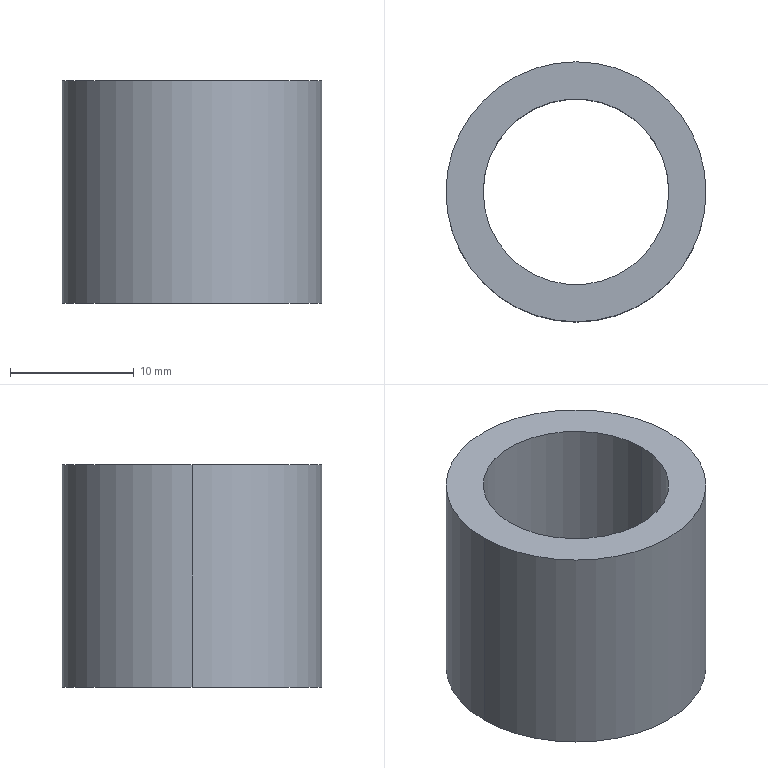Part | NX | features BREP 1 | 1 solid | 6 faces | box 21 x 21 x 18 mm | volume 3054 mm3 | cylinder 4 | plane 2 | commonest cylinder face diameters 15 x2 21 x2
STEP:
#1=CARTESIAN_POINT('',(-7.5,0.,18.));
#2=VERTEX_POINT('',#1);
#3=CARTESIAN_POINT('',(7.5,0.,18.));
#4=VERTEX_POINT('',#3);
#5=CARTESIAN_POINT('',(0.,0.,18.));
#6=DIRECTION('',(0.,0.,1.));
#7=DIRECTION('',(1.,0.,0.));
#8=AXIS2_PLACEMENT_3D('',#5,#6,#7);
#9=CIRCLE('',#8,7.5);
#10=EDGE_CURVE('',#2,#4,#9,.T.);
#11=ORIENTED_EDGE('',*,*,#10,.T.);
#12=CARTESIAN_POINT('',(7.5,0.,0.));
#13=VERTEX_POINT('',#12);
#14=CARTESIAN_POINT('',(7.5,0.,18.));
#15=DIRECTION('',(0.,0.,-1.));
#16=VECTOR('',#15,1000.);
#17=LINE('',#14,#16);
#18=EDGE_CURVE('',#13,#4,#17,.F.);
#19=ORIENTED_EDGE('',*,*,#18,.F.);
#20=CARTESIAN_POINT('',(-7.5,0.,0.));
#21=VERTEX_POINT('',#20);
#22=CARTESIAN_POINT('',(0.,0.,0.));
#23=DIRECTION('',(0.,0.,1.));
#24=DIRECTION('',(1.,0.,0.));
#25=AXIS2_PLACEMENT_3D('',#22,#23,#24);
#26=CIRCLE('',#25,7.5);
#27=EDGE_CURVE('',#21,#13,#26,.T.);
#28=ORIENTED_EDGE('',*,*,#27,.F.);
#29=CARTESIAN_POINT('',(-7.5,0.,18.));
#30=DIRECTION('',(0.,0.,-1.));
#31=VECTOR('',#30,1000.);
#32=LINE('',#29,#31);
#33=EDGE_CURVE('',#21,#2,#32,.F.);
#34=ORIENTED_EDGE('',*,*,#33,.T.);
#35=EDGE_LOOP('',(#11,#19,#28,#34));
#36=FACE_BOUND('',#35,.T.);
#37=CARTESIAN_POINT('',(0.,0.,18.));
#38=DIRECTION('',(0.,0.,-1.));
#39=DIRECTION('',(1.,0.,0.));
#40=AXIS2_PLACEMENT_3D('',#37,#38,#39);
#41=CYLINDRICAL_SURFACE('',#40,7.5);
#42=ADVANCED_FACE('',(#36),#41,.F.);
#43=CARTESIAN_POINT('',(10.5,0.,18.));
#44=VERTEX_POINT('',#43);
#45=CARTESIAN_POINT('',(-10.5,0.,18.));
#46=VERTEX_POINT('',#45);
#47=CARTESIAN_POINT('',(0.,0.,18.));
#48=DIRECTION('',(0.,0.,1.));
#49=DIRECTION('',(1.,0.,0.));
#50=AXIS2_PLACEMENT_3D('',#47,#48,#49);
#51=CIRCLE('',#50,10.5);
#52=EDGE_CURVE('',#44,#46,#51,.T.);
#53=ORIENTED_EDGE('',*,*,#52,.F.);
#54=CARTESIAN_POINT('',(10.5,0.,0.));
#55=VERTEX_POINT('',#54);
#56=CARTESIAN_POINT('',(10.5,0.,18.));
#57=DIRECTION('',(0.,0.,-1.));
#58=VECTOR('',#57,1000.);
#59=LINE('',#56,#58);
#60=EDGE_CURVE('',#55,#44,#59,.F.);
#61=ORIENTED_EDGE('',*,*,#60,.F.);
#62=CARTESIAN_POINT('',(-10.5,0.,0.));
#63=VERTEX_POINT('',#62);
#64=CARTESIAN_POINT('',(0.,0.,0.));
#65=DIRECTION('',(0.,0.,1.));
#66=DIRECTION('',(1.,0.,0.));
#67=AXIS2_PLACEMENT_3D('',#64,#65,#66);
#68=CIRCLE('',#67,10.5);
#69=EDGE_CURVE('',#55,#63,#68,.T.);
#70=ORIENTED_EDGE('',*,*,#69,.T.);
#71=CARTESIAN_POINT('',(-10.5,0.,18.));
#72=DIRECTION('',(0.,0.,-1.));
#73=VECTOR('',#72,1000.);
#74=LINE('',#71,#73);
#75=EDGE_CURVE('',#63,#46,#74,.F.);
#76=ORIENTED_EDGE('',*,*,#75,.T.);
#77=EDGE_LOOP('',(#53,#61,#70,#76));
#78=FACE_BOUND('',#77,.T.);
#79=CARTESIAN_POINT('',(0.,0.,18.));
#80=DIRECTION('',(0.,0.,-1.));
#81=DIRECTION('',(1.,0.,0.));
#82=AXIS2_PLACEMENT_3D('',#79,#80,#81);
#83=CYLINDRICAL_SURFACE('',#82,10.5);
#84=ADVANCED_FACE('',(#78),#83,.T.);
#85=CARTESIAN_POINT('',(0.,0.,18.));
#86=DIRECTION('',(0.,0.,1.));
#87=DIRECTION('',(1.,0.,0.));
#88=AXIS2_PLACEMENT_3D('',#85,#86,#87);
#89=CIRCLE('',#88,10.5);
#90=EDGE_CURVE('',#46,#44,#89,.T.);
#91=ORIENTED_EDGE('',*,*,#90,.T.);
#92=ORIENTED_EDGE('',*,*,#52,.T.);
#93=EDGE_LOOP('',(#91,#92));
#94=FACE_BOUND('',#93,.T.);
#95=ORIENTED_EDGE('',*,*,#10,.F.);
#96=CARTESIAN_POINT('',(0.,0.,18.));
#97=DIRECTION('',(0.,0.,1.));
#98=DIRECTION('',(1.,0.,0.));
#99=AXIS2_PLACEMENT_3D('',#96,#97,#98);
#100=CIRCLE('',#99,7.5);
#101=EDGE_CURVE('',#4,#2,#100,.T.);
#102=ORIENTED_EDGE('',*,*,#101,.F.);
#103=EDGE_LOOP('',(#95,#102));
#104=FACE_BOUND('',#103,.T.);
#105=CARTESIAN_POINT('',(0.,0.,18.));
#106=DIRECTION('',(0.,0.,1.));
#107=DIRECTION('',(-1.,0.,0.));
#108=AXIS2_PLACEMENT_3D('',#105,#106,#107);
#109=PLANE('',#108);
#110=ADVANCED_FACE('',(#94,#104),#109,.T.);
#111=CARTESIAN_POINT('',(0.,0.,0.));
#112=DIRECTION('',(0.,0.,1.));
#113=DIRECTION('',(1.,0.,0.));
#114=AXIS2_PLACEMENT_3D('',#111,#112,#113);
#115=CIRCLE('',#114,10.5);
#116=EDGE_CURVE('',#63,#55,#115,.T.);
#117=ORIENTED_EDGE('',*,*,#116,.F.);
#118=ORIENTED_EDGE('',*,*,#69,.F.);
#119=EDGE_LOOP('',(#117,#118));
#120=FACE_BOUND('',#119,.T.);
#121=ORIENTED_EDGE('',*,*,#27,.T.);
#122=CARTESIAN_POINT('',(0.,0.,0.));
#123=DIRECTION('',(0.,0.,1.));
#124=DIRECTION('',(1.,0.,0.));
#125=AXIS2_PLACEMENT_3D('',#122,#123,#124);
#126=CIRCLE('',#125,7.5);
#127=EDGE_CURVE('',#13,#21,#126,.T.);
#128=ORIENTED_EDGE('',*,*,#127,.T.);
#129=EDGE_LOOP('',(#121,#128));
#130=FACE_BOUND('',#129,.T.);
#131=CARTESIAN_POINT('',(0.,0.,0.));
#132=DIRECTION('',(0.,0.,1.));
#133=DIRECTION('',(-1.,0.,0.));
#134=AXIS2_PLACEMENT_3D('',#131,#132,#133);
#135=PLANE('',#134);
#136=ADVANCED_FACE('',(#120,#130),#135,.F.);
#137=ORIENTED_EDGE('',*,*,#60,.T.);
#138=ORIENTED_EDGE('',*,*,#90,.F.);
#139=ORIENTED_EDGE('',*,*,#75,.F.);
#140=ORIENTED_EDGE('',*,*,#116,.T.);
#141=EDGE_LOOP('',(#137,#138,#139,#140));
#142=FACE_BOUND('',#141,.T.);
#143=CARTESIAN_POINT('',(0.,0.,18.));
#144=DIRECTION('',(0.,0.,-1.));
#145=DIRECTION('',(1.,0.,0.));
#146=AXIS2_PLACEMENT_3D('',#143,#144,#145);
#147=CYLINDRICAL_SURFACE('',#146,10.5);
#148=ADVANCED_FACE('',(#142),#147,.T.);
#149=ORIENTED_EDGE('',*,*,#18,.T.);
#150=ORIENTED_EDGE('',*,*,#101,.T.);
#151=ORIENTED_EDGE('',*,*,#33,.F.);
#152=ORIENTED_EDGE('',*,*,#127,.F.);
#153=EDGE_LOOP('',(#149,#150,#151,#152));
#154=FACE_BOUND('',#153,.T.);
#155=CARTESIAN_POINT('',(0.,0.,18.));
#156=DIRECTION('',(0.,0.,-1.));
#157=DIRECTION('',(1.,0.,0.));
#158=AXIS2_PLACEMENT_3D('',#155,#156,#157);
#159=CYLINDRICAL_SURFACE('',#158,7.5);
#160=ADVANCED_FACE('',(#154),#159,.F.);
#161=CLOSED_SHELL('',(#42,#84,#110,#136,#148,#160));
#162=MANIFOLD_SOLID_BREP('',#161);
#163=(LENGTH_UNIT()NAMED_UNIT(*)SI_UNIT(.MILLI.,.METRE.));
#164=UNCERTAINTY_MEASURE_WITH_UNIT(LENGTH_MEASURE(0.00001),#163,'','');
#165=(NAMED_UNIT(*)PLANE_ANGLE_UNIT()SI_UNIT($,.RADIAN.));
#166=(NAMED_UNIT(*)SI_UNIT($,.STERADIAN.)SOLID_ANGLE_UNIT());
#167=(GEOMETRIC_REPRESENTATION_CONTEXT(3)GLOBAL_UNCERTAINTY_ASSIGNED_CONTEXT((#164))GLOBAL_UNIT_ASSIGNED_CONTEXT((#163,#165,#166))REPRESENTATION_CONTEXT('',''));
#168=ADVANCED_BREP_SHAPE_REPRESENTATION('',(#162),#167);